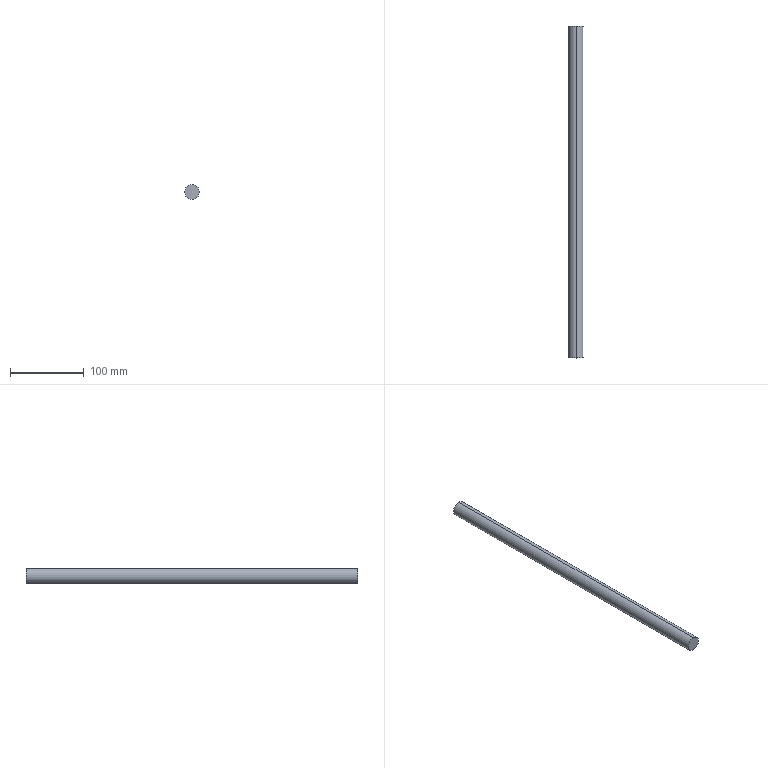Part | STEP file | Plain shaft | 1 solid | 4 faces | box 20 x 450 x 20 mm | volume 141372 mm3 | cylinder 2 | plane 2 | commonest cylinder face diameters 20 x2
STEP:
#1=CARTESIAN_POINT('',(0.,0.,0.));
#2=DIRECTION('',(0.,0.,1.));
#3=DIRECTION('',(1.,0.,0.));
#4=AXIS2_PLACEMENT_3D('',#1,#2,#3);
#5=CARTESIAN_POINT('',(0.,450.,10.));
#6=VERTEX_POINT('',#5);
#7=CARTESIAN_POINT('',(0.,450.,-10.));
#8=VERTEX_POINT('',#7);
#9=CARTESIAN_POINT('',(0.,450.,0.));
#10=DIRECTION('',(0.,1.,0.));
#11=DIRECTION('',(0.,0.,1.));
#12=AXIS2_PLACEMENT_3D('',#9,#10,#11);
#13=CIRCLE('',#12,10.);
#14=CARTESIAN_POINT('',(0.,450.,0.));
#15=DIRECTION('',(0.,-1.,0.));
#16=DIRECTION('',(0.,0.,-1.));
#17=AXIS2_PLACEMENT_3D('',#14,#15,#16);
#18=CYLINDRICAL_SURFACE('',#17,10.);
#19=CARTESIAN_POINT('',(3.142,0.));
#20=DIRECTION('',(-1.,0.));
#21=VECTOR('',#20,1.);
#22=LINE('',#19,#21);
#23=(GEOMETRIC_REPRESENTATION_CONTEXT(2)PARAMETRIC_REPRESENTATION_CONTEXT()REPRESENTATION_CONTEXT('',''));
#24=DEFINITIONAL_REPRESENTATION('',(#22),#23);
#25=PCURVE('',#18,#24);
#26=CARTESIAN_POINT('',(0.,450.,0.));
#27=DIRECTION('',(0.,1.,0.));
#28=DIRECTION('',(0.,0.,1.));
#29=AXIS2_PLACEMENT_3D('',#26,#27,#28);
#30=PLANE('',#29);
#31=CARTESIAN_POINT('',(0.,0.));
#32=DIRECTION('',(1.,0.));
#33=AXIS2_PLACEMENT_2D('',#31,#32);
#34=CIRCLE('',#33,10.);
#35=(GEOMETRIC_REPRESENTATION_CONTEXT(2)PARAMETRIC_REPRESENTATION_CONTEXT()REPRESENTATION_CONTEXT('',''));
#36=DEFINITIONAL_REPRESENTATION('',(#34),#35);
#37=PCURVE('',#30,#36);
#38=SURFACE_CURVE('',#13,(#25,#37),.PCURVE_S1.);
#39=EDGE_CURVE('',#6,#8,#38,.T.);
#40=ORIENTED_EDGE('',*,*,#39,.F.);
#41=CARTESIAN_POINT('',(0.,0.,10.));
#42=VERTEX_POINT('',#41);
#43=CARTESIAN_POINT('',(0.,450.,10.));
#44=DIRECTION('',(0.,-1.,0.));
#45=VECTOR('',#44,1.);
#46=LINE('',#43,#45);
#47=CARTESIAN_POINT('',(3.142,0.));
#48=DIRECTION('',(0.,1.));
#49=VECTOR('',#48,1.);
#50=LINE('',#47,#49);
#51=(GEOMETRIC_REPRESENTATION_CONTEXT(2)PARAMETRIC_REPRESENTATION_CONTEXT()REPRESENTATION_CONTEXT('',''));
#52=DEFINITIONAL_REPRESENTATION('',(#50),#51);
#53=PCURVE('',#18,#52);
#54=CARTESIAN_POINT('',(0.,450.,0.));
#55=DIRECTION('',(0.,-1.,0.));
#56=DIRECTION('',(0.,0.,-1.));
#57=AXIS2_PLACEMENT_3D('',#54,#55,#56);
#58=CYLINDRICAL_SURFACE('',#57,10.);
#59=CARTESIAN_POINT('',(3.142,0.));
#60=DIRECTION('',(0.,1.));
#61=VECTOR('',#60,1.);
#62=LINE('',#59,#61);
#63=(GEOMETRIC_REPRESENTATION_CONTEXT(2)PARAMETRIC_REPRESENTATION_CONTEXT()REPRESENTATION_CONTEXT('',''));
#64=DEFINITIONAL_REPRESENTATION('',(#62),#63);
#65=PCURVE('',#58,#64);
#66=SURFACE_CURVE('',#46,(#53,#65),.PCURVE_S1.);
#67=EDGE_CURVE('',#6,#42,#66,.T.);
#68=ORIENTED_EDGE('',*,*,#67,.T.);
#69=CARTESIAN_POINT('',(0.,0.,-10.));
#70=VERTEX_POINT('',#69);
#71=CARTESIAN_POINT('',(0.,0.,0.));
#72=DIRECTION('',(0.,1.,0.));
#73=DIRECTION('',(0.,0.,1.));
#74=AXIS2_PLACEMENT_3D('',#71,#72,#73);
#75=CIRCLE('',#74,10.);
#76=CARTESIAN_POINT('',(3.142,450.));
#77=DIRECTION('',(-1.,0.));
#78=VECTOR('',#77,1.);
#79=LINE('',#76,#78);
#80=(GEOMETRIC_REPRESENTATION_CONTEXT(2)PARAMETRIC_REPRESENTATION_CONTEXT()REPRESENTATION_CONTEXT('',''));
#81=DEFINITIONAL_REPRESENTATION('',(#79),#80);
#82=PCURVE('',#18,#81);
#83=CARTESIAN_POINT('',(0.,0.,0.));
#84=DIRECTION('',(0.,1.,0.));
#85=DIRECTION('',(0.,0.,1.));
#86=AXIS2_PLACEMENT_3D('',#83,#84,#85);
#87=PLANE('',#86);
#88=CARTESIAN_POINT('',(0.,0.));
#89=DIRECTION('',(1.,0.));
#90=AXIS2_PLACEMENT_2D('',#88,#89);
#91=CIRCLE('',#90,10.);
#92=(GEOMETRIC_REPRESENTATION_CONTEXT(2)PARAMETRIC_REPRESENTATION_CONTEXT()REPRESENTATION_CONTEXT('',''));
#93=DEFINITIONAL_REPRESENTATION('',(#91),#92);
#94=PCURVE('',#87,#93);
#95=SURFACE_CURVE('',#75,(#82,#94),.PCURVE_S1.);
#96=EDGE_CURVE('',#42,#70,#95,.T.);
#97=ORIENTED_EDGE('',*,*,#96,.T.);
#98=CARTESIAN_POINT('',(0.,450.,-10.));
#99=DIRECTION('',(0.,-1.,0.));
#100=VECTOR('',#99,1.);
#101=LINE('',#98,#100);
#102=CARTESIAN_POINT('',(0.,0.));
#103=DIRECTION('',(0.,1.));
#104=VECTOR('',#103,1.);
#105=LINE('',#102,#104);
#106=(GEOMETRIC_REPRESENTATION_CONTEXT(2)PARAMETRIC_REPRESENTATION_CONTEXT()REPRESENTATION_CONTEXT('',''));
#107=DEFINITIONAL_REPRESENTATION('',(#105),#106);
#108=PCURVE('',#18,#107);
#109=CARTESIAN_POINT('',(6.283,0.));
#110=DIRECTION('',(0.,1.));
#111=VECTOR('',#110,1.);
#112=LINE('',#109,#111);
#113=(GEOMETRIC_REPRESENTATION_CONTEXT(2)PARAMETRIC_REPRESENTATION_CONTEXT()REPRESENTATION_CONTEXT('',''));
#114=DEFINITIONAL_REPRESENTATION('',(#112),#113);
#115=PCURVE('',#58,#114);
#116=SURFACE_CURVE('',#101,(#108,#115),.PCURVE_S1.);
#117=EDGE_CURVE('',#8,#70,#116,.T.);
#118=ORIENTED_EDGE('',*,*,#117,.F.);
#119=EDGE_LOOP('',(#40,#68,#97,#118));
#120=FACE_BOUND('',#119,.T.);
#121=ADVANCED_FACE('',(#120),#18,.T.);
#122=ORIENTED_EDGE('',*,*,#67,.F.);
#123=CARTESIAN_POINT('',(0.,450.,0.));
#124=DIRECTION('',(0.,1.,0.));
#125=DIRECTION('',(0.,0.,1.));
#126=AXIS2_PLACEMENT_3D('',#123,#124,#125);
#127=CIRCLE('',#126,10.);
#128=CARTESIAN_POINT('',(9.425,0.));
#129=DIRECTION('',(-1.,0.));
#130=VECTOR('',#129,1.);
#131=LINE('',#128,#130);
#132=(GEOMETRIC_REPRESENTATION_CONTEXT(2)PARAMETRIC_REPRESENTATION_CONTEXT()REPRESENTATION_CONTEXT('',''));
#133=DEFINITIONAL_REPRESENTATION('',(#131),#132);
#134=PCURVE('',#58,#133);
#135=CARTESIAN_POINT('',(0.,0.));
#136=DIRECTION('',(1.,0.));
#137=AXIS2_PLACEMENT_2D('',#135,#136);
#138=CIRCLE('',#137,10.);
#139=(GEOMETRIC_REPRESENTATION_CONTEXT(2)PARAMETRIC_REPRESENTATION_CONTEXT()REPRESENTATION_CONTEXT('',''));
#140=DEFINITIONAL_REPRESENTATION('',(#138),#139);
#141=PCURVE('',#30,#140);
#142=SURFACE_CURVE('',#127,(#134,#141),.PCURVE_S1.);
#143=EDGE_CURVE('',#8,#6,#142,.T.);
#144=ORIENTED_EDGE('',*,*,#143,.F.);
#145=ORIENTED_EDGE('',*,*,#117,.T.);
#146=CARTESIAN_POINT('',(0.,0.,0.));
#147=DIRECTION('',(0.,1.,0.));
#148=DIRECTION('',(0.,0.,1.));
#149=AXIS2_PLACEMENT_3D('',#146,#147,#148);
#150=CIRCLE('',#149,10.);
#151=CARTESIAN_POINT('',(9.425,450.));
#152=DIRECTION('',(-1.,0.));
#153=VECTOR('',#152,1.);
#154=LINE('',#151,#153);
#155=(GEOMETRIC_REPRESENTATION_CONTEXT(2)PARAMETRIC_REPRESENTATION_CONTEXT()REPRESENTATION_CONTEXT('',''));
#156=DEFINITIONAL_REPRESENTATION('',(#154),#155);
#157=PCURVE('',#58,#156);
#158=CARTESIAN_POINT('',(0.,0.));
#159=DIRECTION('',(1.,0.));
#160=AXIS2_PLACEMENT_2D('',#158,#159);
#161=CIRCLE('',#160,10.);
#162=(GEOMETRIC_REPRESENTATION_CONTEXT(2)PARAMETRIC_REPRESENTATION_CONTEXT()REPRESENTATION_CONTEXT('',''));
#163=DEFINITIONAL_REPRESENTATION('',(#161),#162);
#164=PCURVE('',#87,#163);
#165=SURFACE_CURVE('',#150,(#157,#164),.PCURVE_S1.);
#166=EDGE_CURVE('',#70,#42,#165,.T.);
#167=ORIENTED_EDGE('',*,*,#166,.T.);
#168=EDGE_LOOP('',(#122,#144,#145,#167));
#169=FACE_BOUND('',#168,.T.);
#170=ADVANCED_FACE('',(#169),#58,.T.);
#171=ORIENTED_EDGE('',*,*,#143,.T.);
#172=ORIENTED_EDGE('',*,*,#39,.T.);
#173=EDGE_LOOP('',(#171,#172));
#174=FACE_BOUND('',#173,.T.);
#175=ADVANCED_FACE('',(#174),#30,.T.);
#176=ORIENTED_EDGE('',*,*,#166,.F.);
#177=ORIENTED_EDGE('',*,*,#96,.F.);
#178=EDGE_LOOP('',(#176,#177));
#179=FACE_BOUND('',#178,.T.);
#180=ADVANCED_FACE('',(#179),#87,.F.);
#181=CLOSED_SHELL('',(#121,#170,#175,#180));
#182=MANIFOLD_SOLID_BREP('',#181);
#183=(LENGTH_UNIT()NAMED_UNIT(*)SI_UNIT(.MILLI.,.METRE.));
#184=UNCERTAINTY_MEASURE_WITH_UNIT(LENGTH_MEASURE(0.0000001),#183,'','');
#185=(NAMED_UNIT(*)PLANE_ANGLE_UNIT()SI_UNIT($,.RADIAN.));
#186=(NAMED_UNIT(*)SI_UNIT($,.STERADIAN.)SOLID_ANGLE_UNIT());
#187=(GEOMETRIC_REPRESENTATION_CONTEXT(3)GLOBAL_UNCERTAINTY_ASSIGNED_CONTEXT((#184))GLOBAL_UNIT_ASSIGNED_CONTEXT((#183,#185,#186))REPRESENTATION_CONTEXT('',''));
#188=ADVANCED_BREP_SHAPE_REPRESENTATION('',(#4,#182),#187);